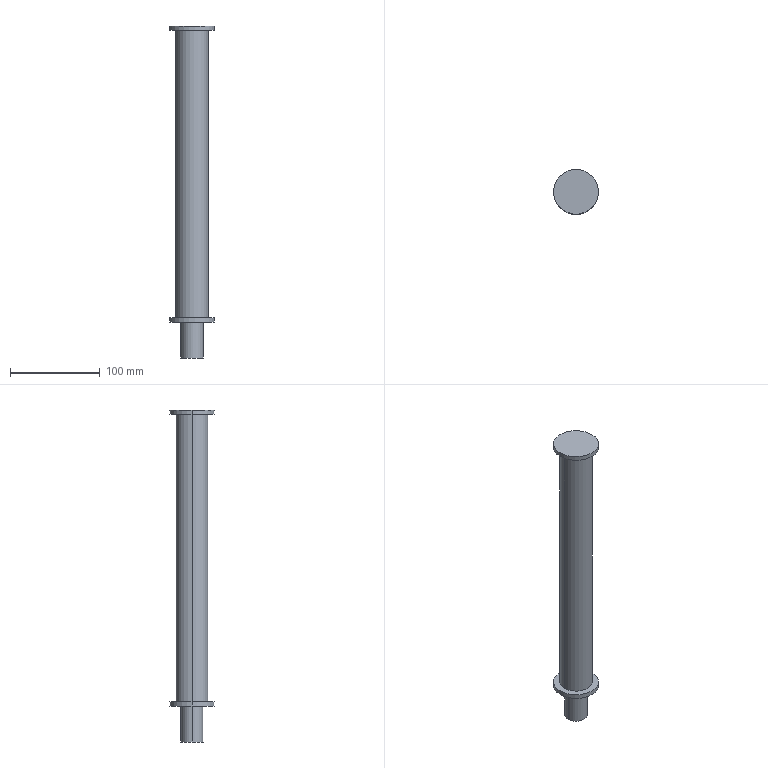Part | STEP file | JUANZHOU_1 | 1 solid | 13 faces | box 50 x 50 x 370 mm | volume 364990 mm3 | cylinder 8 | plane 5 | commonest cylinder face diameters 50 x4 25 x2 36 x2
STEP:
#1=CARTESIAN_POINT('',(0.,0.,0.));
#2=DIRECTION('',(0.,0.,1.));
#3=DIRECTION('',(1.,0.,0.));
#4=AXIS2_PLACEMENT_3D('',#1,#2,#3);
#5=CARTESIAN_POINT('',(18.,0.,-160.));
#6=VERTEX_POINT('',#5);
#7=CARTESIAN_POINT('',(-18.,0.,-160.));
#8=VERTEX_POINT('',#7);
#9=CARTESIAN_POINT('',(0.,0.,-160.));
#10=DIRECTION('',(0.,0.,1.));
#11=DIRECTION('',(1.,0.,0.));
#12=AXIS2_PLACEMENT_3D('',#9,#10,#11);
#13=CIRCLE('',#12,18.);
#14=CARTESIAN_POINT('',(0.,0.,160.));
#15=DIRECTION('',(0.,0.,1.));
#16=DIRECTION('',(1.,0.,0.));
#17=AXIS2_PLACEMENT_3D('',#14,#15,#16);
#18=CYLINDRICAL_SURFACE('',#17,18.);
#19=CARTESIAN_POINT('',(0.,-320.));
#20=DIRECTION('',(1.,0.));
#21=VECTOR('',#20,1.);
#22=LINE('',#19,#21);
#23=(GEOMETRIC_REPRESENTATION_CONTEXT(2)PARAMETRIC_REPRESENTATION_CONTEXT()REPRESENTATION_CONTEXT('',''));
#24=DEFINITIONAL_REPRESENTATION('',(#22),#23);
#25=PCURVE('',#18,#24);
#26=CARTESIAN_POINT('',(0.,0.,-160.));
#27=DIRECTION('',(0.,0.,-1.));
#28=DIRECTION('',(-1.,0.,0.));
#29=AXIS2_PLACEMENT_3D('',#26,#27,#28);
#30=PLANE('',#29);
#31=CARTESIAN_POINT('',(-18.,0.));
#32=CARTESIAN_POINT('',(-18.,31.177));
#33=CARTESIAN_POINT('',(9.,15.588));
#34=CARTESIAN_POINT('',(36.,0.));
#35=CARTESIAN_POINT('',(9.,-15.588));
#36=CARTESIAN_POINT('',(-18.,-31.177));
#37=CARTESIAN_POINT('',(-18.,0.));
#38=(BOUNDED_CURVE()B_SPLINE_CURVE(2,(#31,#32,#33,#34,#35,#36,#37),.UNSPECIFIED.,.T.,.F.)B_SPLINE_CURVE_WITH_KNOTS((1,2,2,2,2,1),(-2.094,0.,2.094,4.189,6.283,8.378),.UNSPECIFIED.)CURVE()GEOMETRIC_REPRESENTATION_ITEM()RATIONAL_B_SPLINE_CURVE((1.,0.5,1.,0.5,1.,0.5,1.))REPRESENTATION_ITEM(''));
#39=(GEOMETRIC_REPRESENTATION_CONTEXT(2)PARAMETRIC_REPRESENTATION_CONTEXT()REPRESENTATION_CONTEXT('',''));
#40=DEFINITIONAL_REPRESENTATION('',(#38),#39);
#41=PCURVE('',#30,#40);
#42=SURFACE_CURVE('',#13,(#25,#41),.PCURVE_S1.);
#43=EDGE_CURVE('',#6,#8,#42,.T.);
#44=ORIENTED_EDGE('',*,*,#43,.T.);
#45=CARTESIAN_POINT('',(-18.,0.,160.));
#46=VERTEX_POINT('',#45);
#47=CARTESIAN_POINT('',(-18.,0.,160.));
#48=DIRECTION('',(0.,0.,1.));
#49=VECTOR('',#48,1.);
#50=LINE('',#47,#49);
#51=CARTESIAN_POINT('',(3.142,0.));
#52=DIRECTION('',(0.,1.));
#53=VECTOR('',#52,1.);
#54=LINE('',#51,#53);
#55=(GEOMETRIC_REPRESENTATION_CONTEXT(2)PARAMETRIC_REPRESENTATION_CONTEXT()REPRESENTATION_CONTEXT('',''));
#56=DEFINITIONAL_REPRESENTATION('',(#54),#55);
#57=PCURVE('',#18,#56);
#58=CARTESIAN_POINT('',(0.,0.,160.));
#59=DIRECTION('',(0.,0.,1.));
#60=DIRECTION('',(1.,0.,0.));
#61=AXIS2_PLACEMENT_3D('',#58,#59,#60);
#62=CYLINDRICAL_SURFACE('',#61,18.);
#63=CARTESIAN_POINT('',(3.142,0.));
#64=DIRECTION('',(0.,1.));
#65=VECTOR('',#64,1.);
#66=LINE('',#63,#65);
#67=(GEOMETRIC_REPRESENTATION_CONTEXT(2)PARAMETRIC_REPRESENTATION_CONTEXT()REPRESENTATION_CONTEXT('',''));
#68=DEFINITIONAL_REPRESENTATION('',(#66),#67);
#69=PCURVE('',#62,#68);
#70=SURFACE_CURVE('',#50,(#57,#69),.PCURVE_S1.);
#71=EDGE_CURVE('',#8,#46,#70,.T.);
#72=ORIENTED_EDGE('',*,*,#71,.T.);
#73=CARTESIAN_POINT('',(18.,0.,160.));
#74=VERTEX_POINT('',#73);
#75=CARTESIAN_POINT('',(0.,0.,160.));
#76=DIRECTION('',(0.,0.,-1.));
#77=DIRECTION('',(1.,0.,0.));
#78=AXIS2_PLACEMENT_3D('',#75,#76,#77);
#79=CIRCLE('',#78,18.);
#80=CARTESIAN_POINT('',(6.283,0.));
#81=DIRECTION('',(-1.,0.));
#82=VECTOR('',#81,1.);
#83=LINE('',#80,#82);
#84=(GEOMETRIC_REPRESENTATION_CONTEXT(2)PARAMETRIC_REPRESENTATION_CONTEXT()REPRESENTATION_CONTEXT('',''));
#85=DEFINITIONAL_REPRESENTATION('',(#83),#84);
#86=PCURVE('',#18,#85);
#87=CARTESIAN_POINT('',(0.,0.,160.));
#88=DIRECTION('',(0.,0.,1.));
#89=DIRECTION('',(1.,0.,0.));
#90=AXIS2_PLACEMENT_3D('',#87,#88,#89);
#91=PLANE('',#90);
#92=CARTESIAN_POINT('',(18.,0.));
#93=CARTESIAN_POINT('',(18.,-31.177));
#94=CARTESIAN_POINT('',(-9.,-15.588));
#95=CARTESIAN_POINT('',(-36.,0.));
#96=CARTESIAN_POINT('',(-9.,15.588));
#97=CARTESIAN_POINT('',(18.,31.177));
#98=CARTESIAN_POINT('',(18.,0.));
#99=(BOUNDED_CURVE()B_SPLINE_CURVE(2,(#92,#93,#94,#95,#96,#97,#98),.UNSPECIFIED.,.T.,.F.)B_SPLINE_CURVE_WITH_KNOTS((1,2,2,2,2,1),(-2.094,0.,2.094,4.189,6.283,8.378),.UNSPECIFIED.)CURVE()GEOMETRIC_REPRESENTATION_ITEM()RATIONAL_B_SPLINE_CURVE((1.,0.5,1.,0.5,1.,0.5,1.))REPRESENTATION_ITEM(''));
#100=(GEOMETRIC_REPRESENTATION_CONTEXT(2)PARAMETRIC_REPRESENTATION_CONTEXT()REPRESENTATION_CONTEXT('',''));
#101=DEFINITIONAL_REPRESENTATION('',(#99),#100);
#102=PCURVE('',#91,#101);
#103=SURFACE_CURVE('',#79,(#86,#102),.PCURVE_S1.);
#104=EDGE_CURVE('',#46,#74,#103,.T.);
#105=ORIENTED_EDGE('',*,*,#104,.T.);
#106=CARTESIAN_POINT('',(18.,0.,160.));
#107=DIRECTION('',(0.,0.,1.));
#108=VECTOR('',#107,1.);
#109=LINE('',#106,#108);
#110=CARTESIAN_POINT('',(0.,0.));
#111=DIRECTION('',(0.,1.));
#112=VECTOR('',#111,1.);
#113=LINE('',#110,#112);
#114=(GEOMETRIC_REPRESENTATION_CONTEXT(2)PARAMETRIC_REPRESENTATION_CONTEXT()REPRESENTATION_CONTEXT('',''));
#115=DEFINITIONAL_REPRESENTATION('',(#113),#114);
#116=PCURVE('',#18,#115);
#117=CARTESIAN_POINT('',(6.283,0.));
#118=DIRECTION('',(0.,1.));
#119=VECTOR('',#118,1.);
#120=LINE('',#117,#119);
#121=(GEOMETRIC_REPRESENTATION_CONTEXT(2)PARAMETRIC_REPRESENTATION_CONTEXT()REPRESENTATION_CONTEXT('',''));
#122=DEFINITIONAL_REPRESENTATION('',(#120),#121);
#123=PCURVE('',#62,#122);
#124=SURFACE_CURVE('',#109,(#116,#123),.PCURVE_S1.);
#125=EDGE_CURVE('',#6,#74,#124,.T.);
#126=ORIENTED_EDGE('',*,*,#125,.F.);
#127=EDGE_LOOP('',(#44,#72,#105,#126));
#128=FACE_BOUND('',#127,.T.);
#129=ADVANCED_FACE('',(#128),#18,.T.);
#130=CARTESIAN_POINT('',(-25.,0.,-160.));
#131=VERTEX_POINT('',#130);
#132=CARTESIAN_POINT('',(25.,0.,-160.));
#133=VERTEX_POINT('',#132);
#134=CARTESIAN_POINT('',(0.,0.,-160.));
#135=DIRECTION('',(0.,0.,-1.));
#136=DIRECTION('',(-1.,0.,0.));
#137=AXIS2_PLACEMENT_3D('',#134,#135,#136);
#138=CIRCLE('',#137,25.);
#139=CARTESIAN_POINT('',(0.,0.,-165.));
#140=DIRECTION('',(0.,0.,-1.));
#141=DIRECTION('',(-1.,0.,0.));
#142=AXIS2_PLACEMENT_3D('',#139,#140,#141);
#143=CYLINDRICAL_SURFACE('',#142,25.);
#144=CARTESIAN_POINT('',(0.,-5.));
#145=DIRECTION('',(1.,0.));
#146=VECTOR('',#145,1.);
#147=LINE('',#144,#146);
#148=(GEOMETRIC_REPRESENTATION_CONTEXT(2)PARAMETRIC_REPRESENTATION_CONTEXT()REPRESENTATION_CONTEXT('',''));
#149=DEFINITIONAL_REPRESENTATION('',(#147),#148);
#150=PCURVE('',#143,#149);
#151=CARTESIAN_POINT('',(0.,0.));
#152=DIRECTION('',(1.,0.));
#153=AXIS2_PLACEMENT_2D('',#151,#152);
#154=CIRCLE('',#153,25.);
#155=(GEOMETRIC_REPRESENTATION_CONTEXT(2)PARAMETRIC_REPRESENTATION_CONTEXT()REPRESENTATION_CONTEXT('',''));
#156=DEFINITIONAL_REPRESENTATION('',(#154),#155);
#157=PCURVE('',#30,#156);
#158=SURFACE_CURVE('',#138,(#150,#157),.PCURVE_S1.);
#159=EDGE_CURVE('',#131,#133,#158,.T.);
#160=ORIENTED_EDGE('',*,*,#159,.T.);
#161=CARTESIAN_POINT('',(25.,0.,-165.));
#162=VERTEX_POINT('',#161);
#163=CARTESIAN_POINT('',(25.,0.,-165.));
#164=DIRECTION('',(0.,0.,-1.));
#165=VECTOR('',#164,1.);
#166=LINE('',#163,#165);
#167=CARTESIAN_POINT('',(3.142,0.));
#168=DIRECTION('',(0.,1.));
#169=VECTOR('',#168,1.);
#170=LINE('',#167,#169);
#171=(GEOMETRIC_REPRESENTATION_CONTEXT(2)PARAMETRIC_REPRESENTATION_CONTEXT()REPRESENTATION_CONTEXT('',''));
#172=DEFINITIONAL_REPRESENTATION('',(#170),#171);
#173=PCURVE('',#143,#172);
#174=CARTESIAN_POINT('',(0.,0.,-165.));
#175=DIRECTION('',(0.,0.,-1.));
#176=DIRECTION('',(-1.,0.,0.));
#177=AXIS2_PLACEMENT_3D('',#174,#175,#176);
#178=CYLINDRICAL_SURFACE('',#177,25.);
#179=CARTESIAN_POINT('',(3.142,0.));
#180=DIRECTION('',(0.,1.));
#181=VECTOR('',#180,1.);
#182=LINE('',#179,#181);
#183=(GEOMETRIC_REPRESENTATION_CONTEXT(2)PARAMETRIC_REPRESENTATION_CONTEXT()REPRESENTATION_CONTEXT('',''));
#184=DEFINITIONAL_REPRESENTATION('',(#182),#183);
#185=PCURVE('',#178,#184);
#186=SURFACE_CURVE('',#166,(#173,#185),.PCURVE_S1.);
#187=EDGE_CURVE('',#133,#162,#186,.T.);
#188=ORIENTED_EDGE('',*,*,#187,.T.);
#189=CARTESIAN_POINT('',(-25.,0.,-165.));
#190=VERTEX_POINT('',#189);
#191=CARTESIAN_POINT('',(0.,0.,-165.));
#192=DIRECTION('',(0.,0.,1.));
#193=DIRECTION('',(-1.,0.,0.));
#194=AXIS2_PLACEMENT_3D('',#191,#192,#193);
#195=CIRCLE('',#194,25.);
#196=CARTESIAN_POINT('',(6.283,0.));
#197=DIRECTION('',(-1.,0.));
#198=VECTOR('',#197,1.);
#199=LINE('',#196,#198);
#200=(GEOMETRIC_REPRESENTATION_CONTEXT(2)PARAMETRIC_REPRESENTATION_CONTEXT()REPRESENTATION_CONTEXT('',''));
#201=DEFINITIONAL_REPRESENTATION('',(#199),#200);
#202=PCURVE('',#143,#201);
#203=CARTESIAN_POINT('',(0.,0.,-165.));
#204=DIRECTION('',(0.,0.,-1.));
#205=DIRECTION('',(-1.,0.,0.));
#206=AXIS2_PLACEMENT_3D('',#203,#204,#205);
#207=PLANE('',#206);
#208=CARTESIAN_POINT('',(25.,0.));
#209=CARTESIAN_POINT('',(25.,-43.301));
#210=CARTESIAN_POINT('',(-12.5,-21.651));
#211=CARTESIAN_POINT('',(-50.,0.));
#212=CARTESIAN_POINT('',(-12.5,21.651));
#213=CARTESIAN_POINT('',(25.,43.301));
#214=CARTESIAN_POINT('',(25.,0.));
#215=(BOUNDED_CURVE()B_SPLINE_CURVE(2,(#208,#209,#210,#211,#212,#213,#214),.UNSPECIFIED.,.T.,.F.)B_SPLINE_CURVE_WITH_KNOTS((1,2,2,2,2,1),(-2.094,0.,2.094,4.189,6.283,8.378),.UNSPECIFIED.)CURVE()GEOMETRIC_REPRESENTATION_ITEM()RATIONAL_B_SPLINE_CURVE((1.,0.5,1.,0.5,1.,0.5,1.))REPRESENTATION_ITEM(''));
#216=(GEOMETRIC_REPRESENTATION_CONTEXT(2)PARAMETRIC_REPRESENTATION_CONTEXT()REPRESENTATION_CONTEXT('',''));
#217=DEFINITIONAL_REPRESENTATION('',(#215),#216);
#218=PCURVE('',#207,#217);
#219=SURFACE_CURVE('',#195,(#202,#218),.PCURVE_S1.);
#220=EDGE_CURVE('',#162,#190,#219,.T.);
#221=ORIENTED_EDGE('',*,*,#220,.T.);
#222=CARTESIAN_POINT('',(-25.,0.,-165.));
#223=DIRECTION('',(0.,0.,-1.));
#224=VECTOR('',#223,1.);
#225=LINE('',#222,#224);
#226=CARTESIAN_POINT('',(0.,0.));
#227=DIRECTION('',(0.,1.));
#228=VECTOR('',#227,1.);
#229=LINE('',#226,#228);
#230=(GEOMETRIC_REPRESENTATION_CONTEXT(2)PARAMETRIC_REPRESENTATION_CONTEXT()REPRESENTATION_CONTEXT('',''));
#231=DEFINITIONAL_REPRESENTATION('',(#229),#230);
#232=PCURVE('',#143,#231);
#233=CARTESIAN_POINT('',(6.283,0.));
#234=DIRECTION('',(0.,1.));
#235=VECTOR('',#234,1.);
#236=LINE('',#233,#235);
#237=(GEOMETRIC_REPRESENTATION_CONTEXT(2)PARAMETRIC_REPRESENTATION_CONTEXT()REPRESENTATION_CONTEXT('',''));
#238=DEFINITIONAL_REPRESENTATION('',(#236),#237);
#239=PCURVE('',#178,#238);
#240=SURFACE_CURVE('',#225,(#232,#239),.PCURVE_S1.);
#241=EDGE_CURVE('',#131,#190,#240,.T.);
#242=ORIENTED_EDGE('',*,*,#241,.F.);
#243=EDGE_LOOP('',(#160,#188,#221,#242));
#244=FACE_BOUND('',#243,.T.);
#245=ADVANCED_FACE('',(#244),#143,.T.);
#246=CARTESIAN_POINT('',(25.,0.,160.));
#247=VERTEX_POINT('',#246);
#248=CARTESIAN_POINT('',(-25.,0.,160.));
#249=VERTEX_POINT('',#248);
#250=CARTESIAN_POINT('',(0.,0.,160.));
#251=DIRECTION('',(0.,0.,1.));
#252=DIRECTION('',(1.,0.,0.));
#253=AXIS2_PLACEMENT_3D('',#250,#251,#252);
#254=CIRCLE('',#253,25.);
#255=CARTESIAN_POINT('',(0.,0.,165.));
#256=DIRECTION('',(0.,0.,1.));
#257=DIRECTION('',(1.,0.,0.));
#258=AXIS2_PLACEMENT_3D('',#255,#256,#257);
#259=CYLINDRICAL_SURFACE('',#258,25.);
#260=CARTESIAN_POINT('',(0.,-5.));
#261=DIRECTION('',(1.,0.));
#262=VECTOR('',#261,1.);
#263=LINE('',#260,#262);
#264=(GEOMETRIC_REPRESENTATION_CONTEXT(2)PARAMETRIC_REPRESENTATION_CONTEXT()REPRESENTATION_CONTEXT('',''));
#265=DEFINITIONAL_REPRESENTATION('',(#263),#264);
#266=PCURVE('',#259,#265);
#267=CARTESIAN_POINT('',(0.,0.));
#268=DIRECTION('',(1.,0.));
#269=AXIS2_PLACEMENT_2D('',#267,#268);
#270=CIRCLE('',#269,25.);
#271=(GEOMETRIC_REPRESENTATION_CONTEXT(2)PARAMETRIC_REPRESENTATION_CONTEXT()REPRESENTATION_CONTEXT('',''));
#272=DEFINITIONAL_REPRESENTATION('',(#270),#271);
#273=PCURVE('',#91,#272);
#274=SURFACE_CURVE('',#254,(#266,#273),.PCURVE_S1.);
#275=EDGE_CURVE('',#247,#249,#274,.T.);
#276=ORIENTED_EDGE('',*,*,#275,.T.);
#277=CARTESIAN_POINT('',(-25.,0.,165.));
#278=VERTEX_POINT('',#277);
#279=CARTESIAN_POINT('',(-25.,0.,165.));
#280=DIRECTION('',(0.,0.,1.));
#281=VECTOR('',#280,1.);
#282=LINE('',#279,#281);
#283=CARTESIAN_POINT('',(3.142,0.));
#284=DIRECTION('',(0.,1.));
#285=VECTOR('',#284,1.);
#286=LINE('',#283,#285);
#287=(GEOMETRIC_REPRESENTATION_CONTEXT(2)PARAMETRIC_REPRESENTATION_CONTEXT()REPRESENTATION_CONTEXT('',''));
#288=DEFINITIONAL_REPRESENTATION('',(#286),#287);
#289=PCURVE('',#259,#288);
#290=CARTESIAN_POINT('',(0.,0.,165.));
#291=DIRECTION('',(0.,0.,1.));
#292=DIRECTION('',(1.,0.,0.));
#293=AXIS2_PLACEMENT_3D('',#290,#291,#292);
#294=CYLINDRICAL_SURFACE('',#293,25.);
#295=CARTESIAN_POINT('',(3.142,0.));
#296=DIRECTION('',(0.,1.));
#297=VECTOR('',#296,1.);
#298=LINE('',#295,#297);
#299=(GEOMETRIC_REPRESENTATION_CONTEXT(2)PARAMETRIC_REPRESENTATION_CONTEXT()REPRESENTATION_CONTEXT('',''));
#300=DEFINITIONAL_REPRESENTATION('',(#298),#299);
#301=PCURVE('',#294,#300);
#302=SURFACE_CURVE('',#282,(#289,#301),.PCURVE_S1.);
#303=EDGE_CURVE('',#249,#278,#302,.T.);
#304=ORIENTED_EDGE('',*,*,#303,.T.);
#305=CARTESIAN_POINT('',(25.,0.,165.));
#306=VERTEX_POINT('',#305);
#307=CARTESIAN_POINT('',(0.,0.,165.));
#308=DIRECTION('',(0.,0.,-1.));
#309=DIRECTION('',(1.,0.,0.));
#310=AXIS2_PLACEMENT_3D('',#307,#308,#309);
#311=CIRCLE('',#310,25.);
#312=CARTESIAN_POINT('',(6.283,0.));
#313=DIRECTION('',(-1.,0.));
#314=VECTOR('',#313,1.);
#315=LINE('',#312,#314);
#316=(GEOMETRIC_REPRESENTATION_CONTEXT(2)PARAMETRIC_REPRESENTATION_CONTEXT()REPRESENTATION_CONTEXT('',''));
#317=DEFINITIONAL_REPRESENTATION('',(#315),#316);
#318=PCURVE('',#259,#317);
#319=CARTESIAN_POINT('',(0.,0.,165.));
#320=DIRECTION('',(0.,0.,1.));
#321=DIRECTION('',(1.,0.,0.));
#322=AXIS2_PLACEMENT_3D('',#319,#320,#321);
#323=PLANE('',#322);
#324=CARTESIAN_POINT('',(25.,0.));
#325=CARTESIAN_POINT('',(25.,-43.301));
#326=CARTESIAN_POINT('',(-12.5,-21.651));
#327=CARTESIAN_POINT('',(-50.,0.));
#328=CARTESIAN_POINT('',(-12.5,21.651));
#329=CARTESIAN_POINT('',(25.,43.301));
#330=CARTESIAN_POINT('',(25.,0.));
#331=(BOUNDED_CURVE()B_SPLINE_CURVE(2,(#324,#325,#326,#327,#328,#329,#330),.UNSPECIFIED.,.T.,.F.)B_SPLINE_CURVE_WITH_KNOTS((1,2,2,2,2,1),(-2.094,0.,2.094,4.189,6.283,8.378),.UNSPECIFIED.)CURVE()GEOMETRIC_REPRESENTATION_ITEM()RATIONAL_B_SPLINE_CURVE((1.,0.5,1.,0.5,1.,0.5,1.))REPRESENTATION_ITEM(''));
#332=(GEOMETRIC_REPRESENTATION_CONTEXT(2)PARAMETRIC_REPRESENTATION_CONTEXT()REPRESENTATION_CONTEXT('',''));
#333=DEFINITIONAL_REPRESENTATION('',(#331),#332);
#334=PCURVE('',#323,#333);
#335=SURFACE_CURVE('',#311,(#318,#334),.PCURVE_S1.);
#336=EDGE_CURVE('',#278,#306,#335,.T.);
#337=ORIENTED_EDGE('',*,*,#336,.T.);
#338=CARTESIAN_POINT('',(25.,0.,165.));
#339=DIRECTION('',(0.,0.,1.));
#340=VECTOR('',#339,1.);
#341=LINE('',#338,#340);
#342=CARTESIAN_POINT('',(0.,0.));
#343=DIRECTION('',(0.,1.));
#344=VECTOR('',#343,1.);
#345=LINE('',#342,#344);
#346=(GEOMETRIC_REPRESENTATION_CONTEXT(2)PARAMETRIC_REPRESENTATION_CONTEXT()REPRESENTATION_CONTEXT('',''));
#347=DEFINITIONAL_REPRESENTATION('',(#345),#346);
#348=PCURVE('',#259,#347);
#349=CARTESIAN_POINT('',(6.283,0.));
#350=DIRECTION('',(0.,1.));
#351=VECTOR('',#350,1.);
#352=LINE('',#349,#351);
#353=(GEOMETRIC_REPRESENTATION_CONTEXT(2)PARAMETRIC_REPRESENTATION_CONTEXT()REPRESENTATION_CONTEXT('',''));
#354=DEFINITIONAL_REPRESENTATION('',(#352),#353);
#355=PCURVE('',#294,#354);
#356=SURFACE_CURVE('',#341,(#348,#355),.PCURVE_S1.);
#357=EDGE_CURVE('',#247,#306,#356,.T.);
#358=ORIENTED_EDGE('',*,*,#357,.F.);
#359=EDGE_LOOP('',(#276,#304,#337,#358));
#360=FACE_BOUND('',#359,.T.);
#361=ADVANCED_FACE('',(#360),#259,.T.);
#362=CARTESIAN_POINT('',(12.5,0.,-165.));
#363=VERTEX_POINT('',#362);
#364=CARTESIAN_POINT('',(-12.5,0.,-165.));
#365=VERTEX_POINT('',#364);
#366=CARTESIAN_POINT('',(0.,0.,-165.));
#367=DIRECTION('',(0.,0.,1.));
#368=DIRECTION('',(-1.,0.,0.));
#369=AXIS2_PLACEMENT_3D('',#366,#367,#368);
#370=CIRCLE('',#369,12.5);
#371=CARTESIAN_POINT('',(0.,0.,-205.));
#372=DIRECTION('',(0.,0.,-1.));
#373=DIRECTION('',(-1.,0.,0.));
#374=AXIS2_PLACEMENT_3D('',#371,#372,#373);
#375=CYLINDRICAL_SURFACE('',#374,12.5);
#376=CARTESIAN_POINT('',(6.283,-40.));
#377=DIRECTION('',(-1.,0.));
#378=VECTOR('',#377,1.);
#379=LINE('',#376,#378);
#380=(GEOMETRIC_REPRESENTATION_CONTEXT(2)PARAMETRIC_REPRESENTATION_CONTEXT()REPRESENTATION_CONTEXT('',''));
#381=DEFINITIONAL_REPRESENTATION('',(#379),#380);
#382=PCURVE('',#375,#381);
#383=CARTESIAN_POINT('',(12.5,0.));
#384=CARTESIAN_POINT('',(12.5,-21.651));
#385=CARTESIAN_POINT('',(-6.25,-10.825));
#386=CARTESIAN_POINT('',(-25.,0.));
#387=CARTESIAN_POINT('',(-6.25,10.825));
#388=CARTESIAN_POINT('',(12.5,21.651));
#389=CARTESIAN_POINT('',(12.5,0.));
#390=(BOUNDED_CURVE()B_SPLINE_CURVE(2,(#383,#384,#385,#386,#387,#388,#389),.UNSPECIFIED.,.T.,.F.)B_SPLINE_CURVE_WITH_KNOTS((1,2,2,2,2,1),(-2.094,0.,2.094,4.189,6.283,8.378),.UNSPECIFIED.)CURVE()GEOMETRIC_REPRESENTATION_ITEM()RATIONAL_B_SPLINE_CURVE((1.,0.5,1.,0.5,1.,0.5,1.))REPRESENTATION_ITEM(''));
#391=(GEOMETRIC_REPRESENTATION_CONTEXT(2)PARAMETRIC_REPRESENTATION_CONTEXT()REPRESENTATION_CONTEXT('',''));
#392=DEFINITIONAL_REPRESENTATION('',(#390),#391);
#393=PCURVE('',#207,#392);
#394=SURFACE_CURVE('',#370,(#382,#393),.PCURVE_S1.);
#395=EDGE_CURVE('',#363,#365,#394,.T.);
#396=ORIENTED_EDGE('',*,*,#395,.F.);
#397=CARTESIAN_POINT('',(12.5,0.,-205.));
#398=VERTEX_POINT('',#397);
#399=CARTESIAN_POINT('',(12.5,0.,-205.));
#400=DIRECTION('',(0.,0.,-1.));
#401=VECTOR('',#400,1.);
#402=LINE('',#399,#401);
#403=CARTESIAN_POINT('',(3.142,0.));
#404=DIRECTION('',(0.,1.));
#405=VECTOR('',#404,1.);
#406=LINE('',#403,#405);
#407=(GEOMETRIC_REPRESENTATION_CONTEXT(2)PARAMETRIC_REPRESENTATION_CONTEXT()REPRESENTATION_CONTEXT('',''));
#408=DEFINITIONAL_REPRESENTATION('',(#406),#407);
#409=PCURVE('',#375,#408);
#410=CARTESIAN_POINT('',(0.,0.,-205.));
#411=DIRECTION('',(0.,0.,-1.));
#412=DIRECTION('',(-1.,0.,0.));
#413=AXIS2_PLACEMENT_3D('',#410,#411,#412);
#414=CYLINDRICAL_SURFACE('',#413,12.5);
#415=CARTESIAN_POINT('',(3.142,0.));
#416=DIRECTION('',(0.,1.));
#417=VECTOR('',#416,1.);
#418=LINE('',#415,#417);
#419=(GEOMETRIC_REPRESENTATION_CONTEXT(2)PARAMETRIC_REPRESENTATION_CONTEXT()REPRESENTATION_CONTEXT('',''));
#420=DEFINITIONAL_REPRESENTATION('',(#418),#419);
#421=PCURVE('',#414,#420);
#422=SURFACE_CURVE('',#402,(#409,#421),.PCURVE_S1.);
#423=EDGE_CURVE('',#363,#398,#422,.T.);
#424=ORIENTED_EDGE('',*,*,#423,.T.);
#425=CARTESIAN_POINT('',(-12.5,0.,-205.));
#426=VERTEX_POINT('',#425);
#427=CARTESIAN_POINT('',(0.,0.,-205.));
#428=DIRECTION('',(0.,0.,1.));
#429=DIRECTION('',(-1.,0.,0.));
#430=AXIS2_PLACEMENT_3D('',#427,#428,#429);
#431=CIRCLE('',#430,12.5);
#432=CARTESIAN_POINT('',(6.283,0.));
#433=DIRECTION('',(-1.,0.));
#434=VECTOR('',#433,1.);
#435=LINE('',#432,#434);
#436=(GEOMETRIC_REPRESENTATION_CONTEXT(2)PARAMETRIC_REPRESENTATION_CONTEXT()REPRESENTATION_CONTEXT('',''));
#437=DEFINITIONAL_REPRESENTATION('',(#435),#436);
#438=PCURVE('',#375,#437);
#439=CARTESIAN_POINT('',(0.,0.,-205.));
#440=DIRECTION('',(0.,0.,-1.));
#441=DIRECTION('',(-1.,0.,0.));
#442=AXIS2_PLACEMENT_3D('',#439,#440,#441);
#443=PLANE('',#442);
#444=CARTESIAN_POINT('',(12.5,0.));
#445=CARTESIAN_POINT('',(12.5,-21.651));
#446=CARTESIAN_POINT('',(-6.25,-10.825));
#447=CARTESIAN_POINT('',(-25.,0.));
#448=CARTESIAN_POINT('',(-6.25,10.825));
#449=CARTESIAN_POINT('',(12.5,21.651));
#450=CARTESIAN_POINT('',(12.5,0.));
#451=(BOUNDED_CURVE()B_SPLINE_CURVE(2,(#444,#445,#446,#447,#448,#449,#450),.UNSPECIFIED.,.T.,.F.)B_SPLINE_CURVE_WITH_KNOTS((1,2,2,2,2,1),(-2.094,0.,2.094,4.189,6.283,8.378),.UNSPECIFIED.)CURVE()GEOMETRIC_REPRESENTATION_ITEM()RATIONAL_B_SPLINE_CURVE((1.,0.5,1.,0.5,1.,0.5,1.))REPRESENTATION_ITEM(''));
#452=(GEOMETRIC_REPRESENTATION_CONTEXT(2)PARAMETRIC_REPRESENTATION_CONTEXT()REPRESENTATION_CONTEXT('',''));
#453=DEFINITIONAL_REPRESENTATION('',(#451),#452);
#454=PCURVE('',#443,#453);
#455=SURFACE_CURVE('',#431,(#438,#454),.PCURVE_S1.);
#456=EDGE_CURVE('',#398,#426,#455,.T.);
#457=ORIENTED_EDGE('',*,*,#456,.T.);
#458=CARTESIAN_POINT('',(-12.5,0.,-205.));
#459=DIRECTION('',(0.,0.,-1.));
#460=VECTOR('',#459,1.);
#461=LINE('',#458,#460);
#462=CARTESIAN_POINT('',(0.,0.));
#463=DIRECTION('',(0.,1.));
#464=VECTOR('',#463,1.);
#465=LINE('',#462,#464);
#466=(GEOMETRIC_REPRESENTATION_CONTEXT(2)PARAMETRIC_REPRESENTATION_CONTEXT()REPRESENTATION_CONTEXT('',''));
#467=DEFINITIONAL_REPRESENTATION('',(#465),#466);
#468=PCURVE('',#375,#467);
#469=CARTESIAN_POINT('',(6.283,0.));
#470=DIRECTION('',(0.,1.));
#471=VECTOR('',#470,1.);
#472=LINE('',#469,#471);
#473=(GEOMETRIC_REPRESENTATION_CONTEXT(2)PARAMETRIC_REPRESENTATION_CONTEXT()REPRESENTATION_CONTEXT('',''));
#474=DEFINITIONAL_REPRESENTATION('',(#472),#473);
#475=PCURVE('',#414,#474);
#476=SURFACE_CURVE('',#461,(#468,#475),.PCURVE_S1.);
#477=EDGE_CURVE('',#365,#426,#476,.T.);
#478=ORIENTED_EDGE('',*,*,#477,.F.);
#479=EDGE_LOOP('',(#396,#424,#457,#478));
#480=FACE_BOUND('',#479,.T.);
#481=ADVANCED_FACE('',(#480),#375,.T.);
#482=ORIENTED_EDGE('',*,*,#71,.F.);
#483=CARTESIAN_POINT('',(0.,0.,-160.));
#484=DIRECTION('',(0.,0.,1.));
#485=DIRECTION('',(1.,0.,0.));
#486=AXIS2_PLACEMENT_3D('',#483,#484,#485);
#487=CIRCLE('',#486,18.);
#488=CARTESIAN_POINT('',(0.,-320.));
#489=DIRECTION('',(1.,0.));
#490=VECTOR('',#489,1.);
#491=LINE('',#488,#490);
#492=(GEOMETRIC_REPRESENTATION_CONTEXT(2)PARAMETRIC_REPRESENTATION_CONTEXT()REPRESENTATION_CONTEXT('',''));
#493=DEFINITIONAL_REPRESENTATION('',(#491),#492);
#494=PCURVE('',#62,#493);
#495=CARTESIAN_POINT('',(-18.,0.));
#496=CARTESIAN_POINT('',(-18.,31.177));
#497=CARTESIAN_POINT('',(9.,15.588));
#498=CARTESIAN_POINT('',(36.,0.));
#499=CARTESIAN_POINT('',(9.,-15.588));
#500=CARTESIAN_POINT('',(-18.,-31.177));
#501=CARTESIAN_POINT('',(-18.,0.));
#502=(BOUNDED_CURVE()B_SPLINE_CURVE(2,(#495,#496,#497,#498,#499,#500,#501),.UNSPECIFIED.,.T.,.F.)B_SPLINE_CURVE_WITH_KNOTS((1,2,2,2,2,1),(-2.094,0.,2.094,4.189,6.283,8.378),.UNSPECIFIED.)CURVE()GEOMETRIC_REPRESENTATION_ITEM()RATIONAL_B_SPLINE_CURVE((1.,0.5,1.,0.5,1.,0.5,1.))REPRESENTATION_ITEM(''));
#503=(GEOMETRIC_REPRESENTATION_CONTEXT(2)PARAMETRIC_REPRESENTATION_CONTEXT()REPRESENTATION_CONTEXT('',''));
#504=DEFINITIONAL_REPRESENTATION('',(#502),#503);
#505=PCURVE('',#30,#504);
#506=SURFACE_CURVE('',#487,(#494,#505),.PCURVE_S1.);
#507=EDGE_CURVE('',#8,#6,#506,.T.);
#508=ORIENTED_EDGE('',*,*,#507,.T.);
#509=ORIENTED_EDGE('',*,*,#125,.T.);
#510=CARTESIAN_POINT('',(0.,0.,160.));
#511=DIRECTION('',(0.,0.,-1.));
#512=DIRECTION('',(1.,0.,0.));
#513=AXIS2_PLACEMENT_3D('',#510,#511,#512);
#514=CIRCLE('',#513,18.);
#515=CARTESIAN_POINT('',(6.283,0.));
#516=DIRECTION('',(-1.,0.));
#517=VECTOR('',#516,1.);
#518=LINE('',#515,#517);
#519=(GEOMETRIC_REPRESENTATION_CONTEXT(2)PARAMETRIC_REPRESENTATION_CONTEXT()REPRESENTATION_CONTEXT('',''));
#520=DEFINITIONAL_REPRESENTATION('',(#518),#519);
#521=PCURVE('',#62,#520);
#522=CARTESIAN_POINT('',(18.,0.));
#523=CARTESIAN_POINT('',(18.,-31.177));
#524=CARTESIAN_POINT('',(-9.,-15.588));
#525=CARTESIAN_POINT('',(-36.,0.));
#526=CARTESIAN_POINT('',(-9.,15.588));
#527=CARTESIAN_POINT('',(18.,31.177));
#528=CARTESIAN_POINT('',(18.,0.));
#529=(BOUNDED_CURVE()B_SPLINE_CURVE(2,(#522,#523,#524,#525,#526,#527,#528),.UNSPECIFIED.,.T.,.F.)B_SPLINE_CURVE_WITH_KNOTS((1,2,2,2,2,1),(-2.094,0.,2.094,4.189,6.283,8.378),.UNSPECIFIED.)CURVE()GEOMETRIC_REPRESENTATION_ITEM()RATIONAL_B_SPLINE_CURVE((1.,0.5,1.,0.5,1.,0.5,1.))REPRESENTATION_ITEM(''));
#530=(GEOMETRIC_REPRESENTATION_CONTEXT(2)PARAMETRIC_REPRESENTATION_CONTEXT()REPRESENTATION_CONTEXT('',''));
#531=DEFINITIONAL_REPRESENTATION('',(#529),#530);
#532=PCURVE('',#91,#531);
#533=SURFACE_CURVE('',#514,(#521,#532),.PCURVE_S1.);
#534=EDGE_CURVE('',#74,#46,#533,.T.);
#535=ORIENTED_EDGE('',*,*,#534,.T.);
#536=EDGE_LOOP('',(#482,#508,#509,#535));
#537=FACE_BOUND('',#536,.T.);
#538=ADVANCED_FACE('',(#537),#62,.T.);
#539=ORIENTED_EDGE('',*,*,#43,.F.);
#540=ORIENTED_EDGE('',*,*,#507,.F.);
#541=EDGE_LOOP('',(#539,#540));
#542=FACE_BOUND('',#541,.T.);
#543=ORIENTED_EDGE('',*,*,#159,.F.);
#544=CARTESIAN_POINT('',(0.,0.,-160.));
#545=DIRECTION('',(0.,0.,-1.));
#546=DIRECTION('',(-1.,0.,0.));
#547=AXIS2_PLACEMENT_3D('',#544,#545,#546);
#548=CIRCLE('',#547,25.);
#549=CARTESIAN_POINT('',(0.,0.));
#550=DIRECTION('',(1.,0.));
#551=AXIS2_PLACEMENT_2D('',#549,#550);
#552=CIRCLE('',#551,25.);
#553=(GEOMETRIC_REPRESENTATION_CONTEXT(2)PARAMETRIC_REPRESENTATION_CONTEXT()REPRESENTATION_CONTEXT('',''));
#554=DEFINITIONAL_REPRESENTATION('',(#552),#553);
#555=PCURVE('',#30,#554);
#556=CARTESIAN_POINT('',(0.,-5.));
#557=DIRECTION('',(1.,0.));
#558=VECTOR('',#557,1.);
#559=LINE('',#556,#558);
#560=(GEOMETRIC_REPRESENTATION_CONTEXT(2)PARAMETRIC_REPRESENTATION_CONTEXT()REPRESENTATION_CONTEXT('',''));
#561=DEFINITIONAL_REPRESENTATION('',(#559),#560);
#562=PCURVE('',#178,#561);
#563=SURFACE_CURVE('',#548,(#555,#562),.PCURVE_S1.);
#564=EDGE_CURVE('',#133,#131,#563,.T.);
#565=ORIENTED_EDGE('',*,*,#564,.F.);
#566=EDGE_LOOP('',(#543,#565));
#567=FACE_BOUND('',#566,.T.);
#568=ADVANCED_FACE('',(#542,#567),#30,.F.);
#569=ORIENTED_EDGE('',*,*,#534,.F.);
#570=ORIENTED_EDGE('',*,*,#104,.F.);
#571=EDGE_LOOP('',(#569,#570));
#572=FACE_BOUND('',#571,.T.);
#573=ORIENTED_EDGE('',*,*,#275,.F.);
#574=CARTESIAN_POINT('',(0.,0.,160.));
#575=DIRECTION('',(0.,0.,1.));
#576=DIRECTION('',(1.,0.,0.));
#577=AXIS2_PLACEMENT_3D('',#574,#575,#576);
#578=CIRCLE('',#577,25.);
#579=CARTESIAN_POINT('',(0.,0.));
#580=DIRECTION('',(1.,0.));
#581=AXIS2_PLACEMENT_2D('',#579,#580);
#582=CIRCLE('',#581,25.);
#583=(GEOMETRIC_REPRESENTATION_CONTEXT(2)PARAMETRIC_REPRESENTATION_CONTEXT()REPRESENTATION_CONTEXT('',''));
#584=DEFINITIONAL_REPRESENTATION('',(#582),#583);
#585=PCURVE('',#91,#584);
#586=CARTESIAN_POINT('',(0.,-5.));
#587=DIRECTION('',(1.,0.));
#588=VECTOR('',#587,1.);
#589=LINE('',#586,#588);
#590=(GEOMETRIC_REPRESENTATION_CONTEXT(2)PARAMETRIC_REPRESENTATION_CONTEXT()REPRESENTATION_CONTEXT('',''));
#591=DEFINITIONAL_REPRESENTATION('',(#589),#590);
#592=PCURVE('',#294,#591);
#593=SURFACE_CURVE('',#578,(#585,#592),.PCURVE_S1.);
#594=EDGE_CURVE('',#249,#247,#593,.T.);
#595=ORIENTED_EDGE('',*,*,#594,.F.);
#596=EDGE_LOOP('',(#573,#595));
#597=FACE_BOUND('',#596,.T.);
#598=ADVANCED_FACE('',(#572,#597),#91,.F.);
#599=ORIENTED_EDGE('',*,*,#187,.F.);
#600=ORIENTED_EDGE('',*,*,#564,.T.);
#601=ORIENTED_EDGE('',*,*,#241,.T.);
#602=CARTESIAN_POINT('',(0.,0.,-165.));
#603=DIRECTION('',(0.,0.,1.));
#604=DIRECTION('',(-1.,0.,0.));
#605=AXIS2_PLACEMENT_3D('',#602,#603,#604);
#606=CIRCLE('',#605,25.);
#607=CARTESIAN_POINT('',(6.283,0.));
#608=DIRECTION('',(-1.,0.));
#609=VECTOR('',#608,1.);
#610=LINE('',#607,#609);
#611=(GEOMETRIC_REPRESENTATION_CONTEXT(2)PARAMETRIC_REPRESENTATION_CONTEXT()REPRESENTATION_CONTEXT('',''));
#612=DEFINITIONAL_REPRESENTATION('',(#610),#611);
#613=PCURVE('',#178,#612);
#614=CARTESIAN_POINT('',(25.,0.));
#615=CARTESIAN_POINT('',(25.,-43.301));
#616=CARTESIAN_POINT('',(-12.5,-21.651));
#617=CARTESIAN_POINT('',(-50.,0.));
#618=CARTESIAN_POINT('',(-12.5,21.651));
#619=CARTESIAN_POINT('',(25.,43.301));
#620=CARTESIAN_POINT('',(25.,0.));
#621=(BOUNDED_CURVE()B_SPLINE_CURVE(2,(#614,#615,#616,#617,#618,#619,#620),.UNSPECIFIED.,.T.,.F.)B_SPLINE_CURVE_WITH_KNOTS((1,2,2,2,2,1),(-2.094,0.,2.094,4.189,6.283,8.378),.UNSPECIFIED.)CURVE()GEOMETRIC_REPRESENTATION_ITEM()RATIONAL_B_SPLINE_CURVE((1.,0.5,1.,0.5,1.,0.5,1.))REPRESENTATION_ITEM(''));
#622=(GEOMETRIC_REPRESENTATION_CONTEXT(2)PARAMETRIC_REPRESENTATION_CONTEXT()REPRESENTATION_CONTEXT('',''));
#623=DEFINITIONAL_REPRESENTATION('',(#621),#622);
#624=PCURVE('',#207,#623);
#625=SURFACE_CURVE('',#606,(#613,#624),.PCURVE_S1.);
#626=EDGE_CURVE('',#190,#162,#625,.T.);
#627=ORIENTED_EDGE('',*,*,#626,.T.);
#628=EDGE_LOOP('',(#599,#600,#601,#627));
#629=FACE_BOUND('',#628,.T.);
#630=ADVANCED_FACE('',(#629),#178,.T.);
#631=ORIENTED_EDGE('',*,*,#303,.F.);
#632=ORIENTED_EDGE('',*,*,#594,.T.);
#633=ORIENTED_EDGE('',*,*,#357,.T.);
#634=CARTESIAN_POINT('',(0.,0.,165.));
#635=DIRECTION('',(0.,0.,-1.));
#636=DIRECTION('',(1.,0.,0.));
#637=AXIS2_PLACEMENT_3D('',#634,#635,#636);
#638=CIRCLE('',#637,25.);
#639=CARTESIAN_POINT('',(6.283,0.));
#640=DIRECTION('',(-1.,0.));
#641=VECTOR('',#640,1.);
#642=LINE('',#639,#641);
#643=(GEOMETRIC_REPRESENTATION_CONTEXT(2)PARAMETRIC_REPRESENTATION_CONTEXT()REPRESENTATION_CONTEXT('',''));
#644=DEFINITIONAL_REPRESENTATION('',(#642),#643);
#645=PCURVE('',#294,#644);
#646=CARTESIAN_POINT('',(25.,0.));
#647=CARTESIAN_POINT('',(25.,-43.301));
#648=CARTESIAN_POINT('',(-12.5,-21.651));
#649=CARTESIAN_POINT('',(-50.,0.));
#650=CARTESIAN_POINT('',(-12.5,21.651));
#651=CARTESIAN_POINT('',(25.,43.301));
#652=CARTESIAN_POINT('',(25.,0.));
#653=(BOUNDED_CURVE()B_SPLINE_CURVE(2,(#646,#647,#648,#649,#650,#651,#652),.UNSPECIFIED.,.T.,.F.)B_SPLINE_CURVE_WITH_KNOTS((1,2,2,2,2,1),(-2.094,0.,2.094,4.189,6.283,8.378),.UNSPECIFIED.)CURVE()GEOMETRIC_REPRESENTATION_ITEM()RATIONAL_B_SPLINE_CURVE((1.,0.5,1.,0.5,1.,0.5,1.))REPRESENTATION_ITEM(''));
#654=(GEOMETRIC_REPRESENTATION_CONTEXT(2)PARAMETRIC_REPRESENTATION_CONTEXT()REPRESENTATION_CONTEXT('',''));
#655=DEFINITIONAL_REPRESENTATION('',(#653),#654);
#656=PCURVE('',#323,#655);
#657=SURFACE_CURVE('',#638,(#645,#656),.PCURVE_S1.);
#658=EDGE_CURVE('',#306,#278,#657,.T.);
#659=ORIENTED_EDGE('',*,*,#658,.T.);
#660=EDGE_LOOP('',(#631,#632,#633,#659));
#661=FACE_BOUND('',#660,.T.);
#662=ADVANCED_FACE('',(#661),#294,.T.);
#663=CARTESIAN_POINT('',(0.,0.,-165.));
#664=DIRECTION('',(0.,0.,1.));
#665=DIRECTION('',(-1.,0.,0.));
#666=AXIS2_PLACEMENT_3D('',#663,#664,#665);
#667=CIRCLE('',#666,12.5);
#668=CARTESIAN_POINT('',(12.5,0.));
#669=CARTESIAN_POINT('',(12.5,-21.651));
#670=CARTESIAN_POINT('',(-6.25,-10.825));
#671=CARTESIAN_POINT('',(-25.,0.));
#672=CARTESIAN_POINT('',(-6.25,10.825));
#673=CARTESIAN_POINT('',(12.5,21.651));
#674=CARTESIAN_POINT('',(12.5,0.));
#675=(BOUNDED_CURVE()B_SPLINE_CURVE(2,(#668,#669,#670,#671,#672,#673,#674),.UNSPECIFIED.,.T.,.F.)B_SPLINE_CURVE_WITH_KNOTS((1,2,2,2,2,1),(-2.094,0.,2.094,4.189,6.283,8.378),.UNSPECIFIED.)CURVE()GEOMETRIC_REPRESENTATION_ITEM()RATIONAL_B_SPLINE_CURVE((1.,0.5,1.,0.5,1.,0.5,1.))REPRESENTATION_ITEM(''));
#676=(GEOMETRIC_REPRESENTATION_CONTEXT(2)PARAMETRIC_REPRESENTATION_CONTEXT()REPRESENTATION_CONTEXT('',''));
#677=DEFINITIONAL_REPRESENTATION('',(#675),#676);
#678=PCURVE('',#207,#677);
#679=CARTESIAN_POINT('',(6.283,-40.));
#680=DIRECTION('',(-1.,0.));
#681=VECTOR('',#680,1.);
#682=LINE('',#679,#681);
#683=(GEOMETRIC_REPRESENTATION_CONTEXT(2)PARAMETRIC_REPRESENTATION_CONTEXT()REPRESENTATION_CONTEXT('',''));
#684=DEFINITIONAL_REPRESENTATION('',(#682),#683);
#685=PCURVE('',#414,#684);
#686=SURFACE_CURVE('',#667,(#678,#685),.PCURVE_S1.);
#687=EDGE_CURVE('',#365,#363,#686,.T.);
#688=ORIENTED_EDGE('',*,*,#687,.T.);
#689=ORIENTED_EDGE('',*,*,#395,.T.);
#690=EDGE_LOOP('',(#688,#689));
#691=FACE_BOUND('',#690,.T.);
#692=ORIENTED_EDGE('',*,*,#626,.F.);
#693=ORIENTED_EDGE('',*,*,#220,.F.);
#694=EDGE_LOOP('',(#692,#693));
#695=FACE_BOUND('',#694,.T.);
#696=ADVANCED_FACE('',(#691,#695),#207,.T.);
#697=ORIENTED_EDGE('',*,*,#658,.F.);
#698=ORIENTED_EDGE('',*,*,#336,.F.);
#699=EDGE_LOOP('',(#697,#698));
#700=FACE_BOUND('',#699,.T.);
#701=ADVANCED_FACE('',(#700),#323,.T.);
#702=ORIENTED_EDGE('',*,*,#423,.F.);
#703=ORIENTED_EDGE('',*,*,#687,.F.);
#704=ORIENTED_EDGE('',*,*,#477,.T.);
#705=CARTESIAN_POINT('',(0.,0.,-205.));
#706=DIRECTION('',(0.,0.,1.));
#707=DIRECTION('',(-1.,0.,0.));
#708=AXIS2_PLACEMENT_3D('',#705,#706,#707);
#709=CIRCLE('',#708,12.5);
#710=CARTESIAN_POINT('',(6.283,0.));
#711=DIRECTION('',(-1.,0.));
#712=VECTOR('',#711,1.);
#713=LINE('',#710,#712);
#714=(GEOMETRIC_REPRESENTATION_CONTEXT(2)PARAMETRIC_REPRESENTATION_CONTEXT()REPRESENTATION_CONTEXT('',''));
#715=DEFINITIONAL_REPRESENTATION('',(#713),#714);
#716=PCURVE('',#414,#715);
#717=CARTESIAN_POINT('',(12.5,0.));
#718=CARTESIAN_POINT('',(12.5,-21.651));
#719=CARTESIAN_POINT('',(-6.25,-10.825));
#720=CARTESIAN_POINT('',(-25.,0.));
#721=CARTESIAN_POINT('',(-6.25,10.825));
#722=CARTESIAN_POINT('',(12.5,21.651));
#723=CARTESIAN_POINT('',(12.5,0.));
#724=(BOUNDED_CURVE()B_SPLINE_CURVE(2,(#717,#718,#719,#720,#721,#722,#723),.UNSPECIFIED.,.T.,.F.)B_SPLINE_CURVE_WITH_KNOTS((1,2,2,2,2,1),(-2.094,0.,2.094,4.189,6.283,8.378),.UNSPECIFIED.)CURVE()GEOMETRIC_REPRESENTATION_ITEM()RATIONAL_B_SPLINE_CURVE((1.,0.5,1.,0.5,1.,0.5,1.))REPRESENTATION_ITEM(''));
#725=(GEOMETRIC_REPRESENTATION_CONTEXT(2)PARAMETRIC_REPRESENTATION_CONTEXT()REPRESENTATION_CONTEXT('',''));
#726=DEFINITIONAL_REPRESENTATION('',(#724),#725);
#727=PCURVE('',#443,#726);
#728=SURFACE_CURVE('',#709,(#716,#727),.PCURVE_S1.);
#729=EDGE_CURVE('',#426,#398,#728,.T.);
#730=ORIENTED_EDGE('',*,*,#729,.T.);
#731=EDGE_LOOP('',(#702,#703,#704,#730));
#732=FACE_BOUND('',#731,.T.);
#733=ADVANCED_FACE('',(#732),#414,.T.);
#734=ORIENTED_EDGE('',*,*,#729,.F.);
#735=ORIENTED_EDGE('',*,*,#456,.F.);
#736=EDGE_LOOP('',(#734,#735));
#737=FACE_BOUND('',#736,.T.);
#738=ADVANCED_FACE('',(#737),#443,.T.);
#739=CLOSED_SHELL('',(#129,#245,#361,#481,#538,#568,#598,#630,#662,#696,#701,#733,#738));
#740=MANIFOLD_SOLID_BREP('',#739);
#741=(LENGTH_UNIT()NAMED_UNIT(*)SI_UNIT(.MILLI.,.METRE.));
#742=UNCERTAINTY_MEASURE_WITH_UNIT(LENGTH_MEASURE(0.0000001),#741,'','');
#743=(NAMED_UNIT(*)PLANE_ANGLE_UNIT()SI_UNIT($,.RADIAN.));
#744=(NAMED_UNIT(*)SI_UNIT($,.STERADIAN.)SOLID_ANGLE_UNIT());
#745=(GEOMETRIC_REPRESENTATION_CONTEXT(3)GLOBAL_UNCERTAINTY_ASSIGNED_CONTEXT((#742))GLOBAL_UNIT_ASSIGNED_CONTEXT((#741,#743,#744))REPRESENTATION_CONTEXT('',''));
#746=ADVANCED_BREP_SHAPE_REPRESENTATION('',(#4,#740),#745);